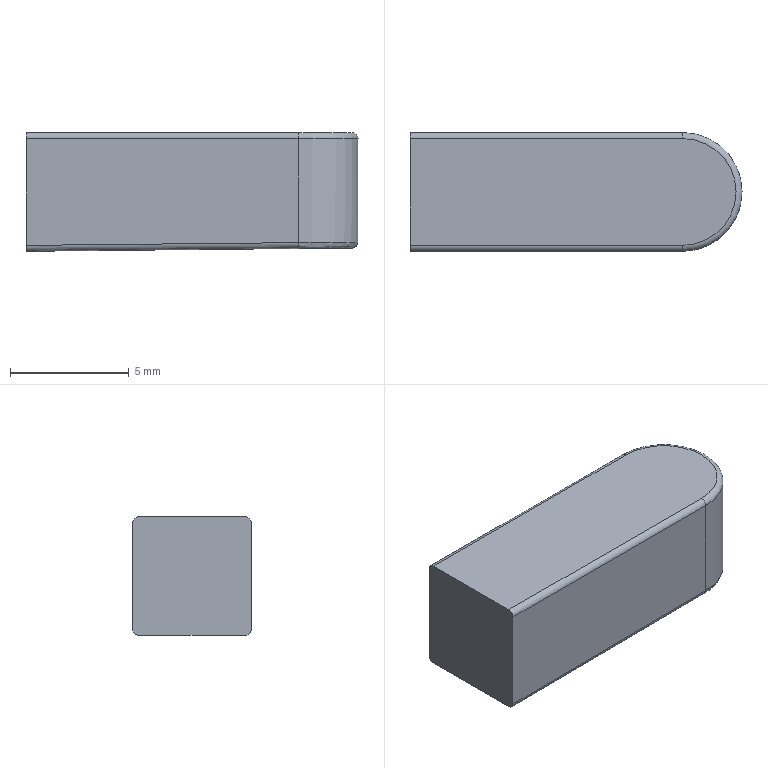Part | SolidWorks | features Cut 1, Extrusion 1, Fillet 1 | 1 solid | 12 faces | box 14 x 5 x 5 mm | volume 331.224 mm3 | plane 5 | cylinder 5 | torus 1 | spline 1 | commonest cylinder face diameters 0.5 x4 5 x1
STEP:
#1=CARTESIAN_POINT('',(-7.,-2.5,4.75));
#2=VERTEX_POINT('',#1);
#3=CARTESIAN_POINT('',(-7.,-2.5,0.25));
#4=VERTEX_POINT('',#3);
#5=CARTESIAN_POINT('',(-7.,-2.5,5.));
#6=DIRECTION('',(0.,0.,-1.));
#7=VECTOR('',#6,1000.);
#8=LINE('',#5,#7);
#9=EDGE_CURVE('',#2,#4,#8,.T.);
#10=ORIENTED_EDGE('',*,*,#9,.F.);
#11=CARTESIAN_POINT('',(-7.,-2.25,5.));
#12=VERTEX_POINT('',#11);
#13=CARTESIAN_POINT('',(-7.,-2.25,4.75));
#14=DIRECTION('',(-1.,0.,0.));
#15=DIRECTION('',(0.,0.,-1.));
#16=AXIS2_PLACEMENT_3D('',#13,#14,#15);
#17=CIRCLE('',#16,0.25);
#18=EDGE_CURVE('',#2,#12,#17,.T.);
#19=ORIENTED_EDGE('',*,*,#18,.T.);
#20=CARTESIAN_POINT('',(-7.,2.25,5.));
#21=VERTEX_POINT('',#20);
#22=CARTESIAN_POINT('',(-7.,2.5,5.));
#23=DIRECTION('',(0.,-1.,0.));
#24=VECTOR('',#23,1000.);
#25=LINE('',#22,#24);
#26=EDGE_CURVE('',#21,#12,#25,.T.);
#27=ORIENTED_EDGE('',*,*,#26,.F.);
#28=CARTESIAN_POINT('',(-7.,2.5,4.75));
#29=VERTEX_POINT('',#28);
#30=CARTESIAN_POINT('',(-7.,2.25,4.75));
#31=DIRECTION('',(-1.,0.,0.));
#32=DIRECTION('',(0.,0.,-1.));
#33=AXIS2_PLACEMENT_3D('',#30,#31,#32);
#34=CIRCLE('',#33,0.25);
#35=EDGE_CURVE('',#21,#29,#34,.T.);
#36=ORIENTED_EDGE('',*,*,#35,.T.);
#37=CARTESIAN_POINT('',(-7.,2.5,0.25));
#38=VERTEX_POINT('',#37);
#39=CARTESIAN_POINT('',(-7.,2.5,5.));
#40=DIRECTION('',(0.,0.,-1.));
#41=VECTOR('',#40,1000.);
#42=LINE('',#39,#41);
#43=EDGE_CURVE('',#29,#38,#42,.T.);
#44=ORIENTED_EDGE('',*,*,#43,.T.);
#45=CARTESIAN_POINT('',(-7.,2.25,0.));
#46=VERTEX_POINT('',#45);
#47=CARTESIAN_POINT('',(-7.,2.5,0.25));
#48=CARTESIAN_POINT('',(-7.,2.5,0.1036));
#49=CARTESIAN_POINT('',(-7.,2.396,0.));
#50=CARTESIAN_POINT('',(-7.,2.25,0.));
#51=(BOUNDED_CURVE()B_SPLINE_CURVE(3,(#47,#48,#49,#50),.UNSPECIFIED.,.F.,.T.)B_SPLINE_CURVE_WITH_KNOTS((4,4),(1.571,3.142),.UNSPECIFIED.)CURVE()GEOMETRIC_REPRESENTATION_ITEM()RATIONAL_B_SPLINE_CURVE((1.,0.8047,0.8047,1.))REPRESENTATION_ITEM(''));
#52=EDGE_CURVE('',#38,#46,#51,.T.);
#53=ORIENTED_EDGE('',*,*,#52,.T.);
#54=CARTESIAN_POINT('',(-7.,-2.25,0.));
#55=VERTEX_POINT('',#54);
#56=CARTESIAN_POINT('',(-7.,2.5,0.));
#57=DIRECTION('',(0.,-1.,0.));
#58=VECTOR('',#57,1000.);
#59=LINE('',#56,#58);
#60=EDGE_CURVE('',#46,#55,#59,.T.);
#61=ORIENTED_EDGE('',*,*,#60,.T.);
#62=CARTESIAN_POINT('',(-7.,-2.25,0.));
#63=CARTESIAN_POINT('',(-7.,-2.396,0.));
#64=CARTESIAN_POINT('',(-7.,-2.5,0.1036));
#65=CARTESIAN_POINT('',(-7.,-2.5,0.25));
#66=(BOUNDED_CURVE()B_SPLINE_CURVE(3,(#62,#63,#64,#65),.UNSPECIFIED.,.F.,.T.)B_SPLINE_CURVE_WITH_KNOTS((4,4),(3.142,4.712),.UNSPECIFIED.)CURVE()GEOMETRIC_REPRESENTATION_ITEM()RATIONAL_B_SPLINE_CURVE((1.,0.8047,0.8047,1.))REPRESENTATION_ITEM(''));
#67=EDGE_CURVE('',#55,#4,#66,.T.);
#68=ORIENTED_EDGE('',*,*,#67,.T.);
#69=EDGE_LOOP('',(#10,#19,#27,#36,#44,#53,#61,#68));
#70=FACE_OUTER_BOUND('',#69,.T.);
#71=CARTESIAN_POINT('',(-7.,2.5,5.));
#72=DIRECTION('',(1.,0.,0.));
#73=DIRECTION('',(0.,0.,-1.));
#74=AXIS2_PLACEMENT_3D('',#71,#72,#73);
#75=PLANE('',#74);
#76=ADVANCED_FACE('',(#70),#75,.F.);
#77=CARTESIAN_POINT('',(4.5,-2.5,4.75));
#78=VERTEX_POINT('',#77);
#79=CARTESIAN_POINT('',(4.5,-2.5,0.365));
#80=VERTEX_POINT('',#79);
#81=CARTESIAN_POINT('',(4.5,-2.5,5.));
#82=DIRECTION('',(0.,0.,-1.));
#83=VECTOR('',#82,1000.);
#84=LINE('',#81,#83);
#85=EDGE_CURVE('',#78,#80,#84,.T.);
#86=ORIENTED_EDGE('',*,*,#85,.F.);
#87=CARTESIAN_POINT('',(4.5,-2.5,4.75));
#88=DIRECTION('',(-1.,0.,0.));
#89=VECTOR('',#88,1000.);
#90=LINE('',#87,#89);
#91=EDGE_CURVE('',#78,#2,#90,.T.);
#92=ORIENTED_EDGE('',*,*,#91,.T.);
#93=ORIENTED_EDGE('',*,*,#9,.T.);
#94=CARTESIAN_POINT('',(4.546,-2.5,0.3655));
#95=DIRECTION('',(1.,0.,0.01));
#96=VECTOR('',#95,1000.);
#97=LINE('',#94,#96);
#98=EDGE_CURVE('',#4,#80,#97,.T.);
#99=ORIENTED_EDGE('',*,*,#98,.T.);
#100=EDGE_LOOP('',(#86,#92,#93,#99));
#101=FACE_OUTER_BOUND('',#100,.T.);
#102=CARTESIAN_POINT('',(4.5,-2.5,5.));
#103=DIRECTION('',(0.,1.,0.));
#104=DIRECTION('',(-1.,0.,0.));
#105=AXIS2_PLACEMENT_3D('',#102,#103,#104);
#106=PLANE('',#105);
#107=ADVANCED_FACE('',(#101),#106,.F.);
#108=CARTESIAN_POINT('',(4.5,2.5,4.75));
#109=VERTEX_POINT('',#108);
#110=CARTESIAN_POINT('',(4.5,2.5,0.365));
#111=VERTEX_POINT('',#110);
#112=CARTESIAN_POINT('',(4.5,2.5,5.));
#113=DIRECTION('',(0.,0.,-1.));
#114=VECTOR('',#113,1000.);
#115=LINE('',#112,#114);
#116=EDGE_CURVE('',#109,#111,#115,.T.);
#117=ORIENTED_EDGE('',*,*,#116,.F.);
#118=CARTESIAN_POINT('',(4.5,0.,4.75));
#119=DIRECTION('',(0.,0.,-1.));
#120=DIRECTION('',(-1.,0.,0.));
#121=AXIS2_PLACEMENT_3D('',#118,#119,#120);
#122=CIRCLE('',#121,2.5);
#123=EDGE_CURVE('',#109,#78,#122,.T.);
#124=ORIENTED_EDGE('',*,*,#123,.T.);
#125=ORIENTED_EDGE('',*,*,#85,.T.);
#126=CARTESIAN_POINT('',(4.5,-2.5,0.365));
#127=CARTESIAN_POINT('',(9.5,-2.5,0.41));
#128=CARTESIAN_POINT('',(9.5,2.5,0.41));
#129=CARTESIAN_POINT('',(4.5,2.5,0.365));
#130=(BOUNDED_CURVE()B_SPLINE_CURVE(3,(#126,#127,#128,#129),.UNSPECIFIED.,.F.,.F.)B_SPLINE_CURVE_WITH_KNOTS((4,4),(1.571,4.712),.UNSPECIFIED.)CURVE()GEOMETRIC_REPRESENTATION_ITEM()RATIONAL_B_SPLINE_CURVE((1.,0.3333,0.3333,1.))REPRESENTATION_ITEM(''));
#131=EDGE_CURVE('',#80,#111,#130,.T.);
#132=ORIENTED_EDGE('',*,*,#131,.T.);
#133=EDGE_LOOP('',(#117,#124,#125,#132));
#134=FACE_OUTER_BOUND('',#133,.T.);
#135=CARTESIAN_POINT('',(4.5,0.,5.));
#136=DIRECTION('',(0.,0.,-1.));
#137=DIRECTION('',(-1.,0.,0.));
#138=AXIS2_PLACEMENT_3D('',#135,#136,#137);
#139=CYLINDRICAL_SURFACE('',#138,2.5);
#140=ADVANCED_FACE('',(#134),#139,.T.);
#141=ORIENTED_EDGE('',*,*,#116,.T.);
#142=CARTESIAN_POINT('',(-6.953,2.5,0.2505));
#143=DIRECTION('',(-1.,0.,-0.01));
#144=VECTOR('',#143,1000.);
#145=LINE('',#142,#144);
#146=EDGE_CURVE('',#111,#38,#145,.T.);
#147=ORIENTED_EDGE('',*,*,#146,.T.);
#148=ORIENTED_EDGE('',*,*,#43,.F.);
#149=CARTESIAN_POINT('',(-7.,2.5,4.75));
#150=DIRECTION('',(1.,0.,0.));
#151=VECTOR('',#150,1000.);
#152=LINE('',#149,#151);
#153=EDGE_CURVE('',#29,#109,#152,.T.);
#154=ORIENTED_EDGE('',*,*,#153,.T.);
#155=EDGE_LOOP('',(#141,#147,#148,#154));
#156=FACE_OUTER_BOUND('',#155,.T.);
#157=CARTESIAN_POINT('',(-7.,2.5,5.));
#158=DIRECTION('',(0.,-1.,0.));
#159=DIRECTION('',(1.,0.,0.));
#160=AXIS2_PLACEMENT_3D('',#157,#158,#159);
#161=PLANE('',#160);
#162=ADVANCED_FACE('',(#156),#161,.F.);
#163=ORIENTED_EDGE('',*,*,#26,.T.);
#164=CARTESIAN_POINT('',(4.5,-2.25,5.));
#165=VERTEX_POINT('',#164);
#166=CARTESIAN_POINT('',(4.5,-2.25,5.));
#167=DIRECTION('',(1.,0.,0.));
#168=VECTOR('',#167,1000.);
#169=LINE('',#166,#168);
#170=EDGE_CURVE('',#12,#165,#169,.T.);
#171=ORIENTED_EDGE('',*,*,#170,.T.);
#172=CARTESIAN_POINT('',(4.5,2.25,5.));
#173=VERTEX_POINT('',#172);
#174=CARTESIAN_POINT('',(4.5,0.,5.));
#175=DIRECTION('',(0.,0.,1.));
#176=DIRECTION('',(-1.,0.,0.));
#177=AXIS2_PLACEMENT_3D('',#174,#175,#176);
#178=CIRCLE('',#177,2.25);
#179=EDGE_CURVE('',#165,#173,#178,.T.);
#180=ORIENTED_EDGE('',*,*,#179,.T.);
#181=CARTESIAN_POINT('',(4.5,2.25,5.));
#182=DIRECTION('',(-1.,0.,0.));
#183=VECTOR('',#182,1000.);
#184=LINE('',#181,#183);
#185=EDGE_CURVE('',#173,#21,#184,.T.);
#186=ORIENTED_EDGE('',*,*,#185,.T.);
#187=EDGE_LOOP('',(#163,#171,#180,#186));
#188=FACE_OUTER_BOUND('',#187,.T.);
#189=CARTESIAN_POINT('',(4.5,0.,5.));
#190=DIRECTION('',(0.,0.,-1.));
#191=DIRECTION('',(-1.,0.,0.));
#192=AXIS2_PLACEMENT_3D('',#189,#190,#191);
#193=PLANE('',#192);
#194=ADVANCED_FACE('',(#188),#193,.F.);
#195=ORIENTED_EDGE('',*,*,#60,.F.);
#196=CARTESIAN_POINT('',(4.502,2.25,0.115));
#197=VERTEX_POINT('',#196);
#198=CARTESIAN_POINT('',(-7.,2.25,0.));
#199=DIRECTION('',(1.,0.,0.01));
#200=VECTOR('',#199,1000.);
#201=LINE('',#198,#200);
#202=EDGE_CURVE('',#46,#197,#201,.T.);
#203=ORIENTED_EDGE('',*,*,#202,.T.);
#204=CARTESIAN_POINT('',(4.502,-2.25,0.115));
#205=VERTEX_POINT('',#204);
#206=CARTESIAN_POINT('',(4.502,2.25,0.115));
#207=CARTESIAN_POINT('',(9.002,2.25,0.16));
#208=CARTESIAN_POINT('',(9.002,-2.25,0.16));
#209=CARTESIAN_POINT('',(4.502,-2.25,0.115));
#210=(BOUNDED_CURVE()B_SPLINE_CURVE(3,(#206,#207,#208,#209),.UNSPECIFIED.,.F.,.T.)B_SPLINE_CURVE_WITH_KNOTS((4,4),(1.571,4.712),.UNSPECIFIED.)CURVE()GEOMETRIC_REPRESENTATION_ITEM()RATIONAL_B_SPLINE_CURVE((1.,0.3333,0.3333,1.))REPRESENTATION_ITEM(''));
#211=EDGE_CURVE('',#197,#205,#210,.T.);
#212=ORIENTED_EDGE('',*,*,#211,.T.);
#213=CARTESIAN_POINT('',(-7.,-2.25,0.));
#214=DIRECTION('',(-1.,0.,-0.01));
#215=VECTOR('',#214,1000.);
#216=LINE('',#213,#215);
#217=EDGE_CURVE('',#205,#55,#216,.T.);
#218=ORIENTED_EDGE('',*,*,#217,.T.);
#219=EDGE_LOOP('',(#195,#203,#212,#218));
#220=FACE_OUTER_BOUND('',#219,.T.);
#221=CARTESIAN_POINT('',(-7.,-2.5,0.));
#222=DIRECTION('',(-0.01,0.,1.));
#223=DIRECTION('',(1.,0.,0.01));
#224=AXIS2_PLACEMENT_3D('',#221,#222,#223);
#225=PLANE('',#224);
#226=ADVANCED_FACE('',(#220),#225,.F.);
#227=ORIENTED_EDGE('',*,*,#35,.F.);
#228=ORIENTED_EDGE('',*,*,#185,.F.);
#229=CARTESIAN_POINT('',(4.5,2.25,4.75));
#230=DIRECTION('',(1.,0.,0.));
#231=DIRECTION('',(0.,0.,-1.));
#232=AXIS2_PLACEMENT_3D('',#229,#230,#231);
#233=CIRCLE('',#232,0.25);
#234=EDGE_CURVE('',#109,#173,#233,.T.);
#235=ORIENTED_EDGE('',*,*,#234,.F.);
#236=ORIENTED_EDGE('',*,*,#153,.F.);
#237=EDGE_LOOP('',(#227,#228,#235,#236));
#238=FACE_OUTER_BOUND('',#237,.T.);
#239=CARTESIAN_POINT('',(4.5,2.25,4.75));
#240=DIRECTION('',(-1.,0.,0.));
#241=DIRECTION('',(0.,-1.,0.));
#242=AXIS2_PLACEMENT_3D('',#239,#240,#241);
#243=CYLINDRICAL_SURFACE('',#242,0.25);
#244=ADVANCED_FACE('',(#238),#243,.T.);
#245=ORIENTED_EDGE('',*,*,#234,.T.);
#246=ORIENTED_EDGE('',*,*,#179,.F.);
#247=CARTESIAN_POINT('',(4.5,-2.25,4.75));
#248=DIRECTION('',(-1.,0.,0.));
#249=DIRECTION('',(0.,0.,1.));
#250=AXIS2_PLACEMENT_3D('',#247,#248,#249);
#251=CIRCLE('',#250,0.25);
#252=EDGE_CURVE('',#78,#165,#251,.T.);
#253=ORIENTED_EDGE('',*,*,#252,.F.);
#254=ORIENTED_EDGE('',*,*,#123,.F.);
#255=EDGE_LOOP('',(#245,#246,#253,#254));
#256=FACE_OUTER_BOUND('',#255,.T.);
#257=CARTESIAN_POINT('',(4.5,0.,4.75));
#258=DIRECTION('',(0.,0.,-1.));
#259=DIRECTION('',(-1.,0.,0.));
#260=AXIS2_PLACEMENT_3D('',#257,#258,#259);
#261=TOROIDAL_SURFACE('',#260,2.25,0.25);
#262=ADVANCED_FACE('',(#256),#261,.T.);
#263=ORIENTED_EDGE('',*,*,#18,.F.);
#264=ORIENTED_EDGE('',*,*,#91,.F.);
#265=ORIENTED_EDGE('',*,*,#252,.T.);
#266=ORIENTED_EDGE('',*,*,#170,.F.);
#267=EDGE_LOOP('',(#263,#264,#265,#266));
#268=FACE_OUTER_BOUND('',#267,.T.);
#269=CARTESIAN_POINT('',(4.5,-2.25,4.75));
#270=DIRECTION('',(1.,0.,0.));
#271=DIRECTION('',(0.,1.,0.));
#272=AXIS2_PLACEMENT_3D('',#269,#270,#271);
#273=CYLINDRICAL_SURFACE('',#272,0.25);
#274=ADVANCED_FACE('',(#268),#273,.T.);
#275=ORIENTED_EDGE('',*,*,#67,.F.);
#276=ORIENTED_EDGE('',*,*,#217,.F.);
#277=CARTESIAN_POINT('',(4.5,-2.25,0.365));
#278=DIRECTION('',(1.,0.,0.01));
#279=DIRECTION('',(0.01,0.,-1.));
#280=AXIS2_PLACEMENT_3D('',#277,#278,#279);
#281=CIRCLE('',#280,0.25);
#282=EDGE_CURVE('',#80,#205,#281,.T.);
#283=ORIENTED_EDGE('',*,*,#282,.F.);
#284=ORIENTED_EDGE('',*,*,#98,.F.);
#285=EDGE_LOOP('',(#275,#276,#283,#284));
#286=FACE_OUTER_BOUND('',#285,.T.);
#287=CARTESIAN_POINT('',(4.546,-2.25,0.3655));
#288=DIRECTION('',(1.,0.,0.01));
#289=DIRECTION('',(0.01,0.,-1.));
#290=AXIS2_PLACEMENT_3D('',#287,#288,#289);
#291=CYLINDRICAL_SURFACE('',#290,0.25);
#292=ADVANCED_FACE('',(#286),#291,.T.);
#293=ORIENTED_EDGE('',*,*,#282,.T.);
#294=ORIENTED_EDGE('',*,*,#211,.F.);
#295=CARTESIAN_POINT('',(4.5,2.25,0.365));
#296=DIRECTION('',(-1.,0.,-0.01));
#297=DIRECTION('',(-0.01,0.,1.));
#298=AXIS2_PLACEMENT_3D('',#295,#296,#297);
#299=CIRCLE('',#298,0.25);
#300=EDGE_CURVE('',#111,#197,#299,.T.);
#301=ORIENTED_EDGE('',*,*,#300,.F.);
#302=ORIENTED_EDGE('',*,*,#131,.F.);
#303=EDGE_LOOP('',(#293,#294,#301,#302));
#304=FACE_OUTER_BOUND('',#303,.T.);
#305=CARTESIAN_POINT('',(4.502,-2.25,0.115));
#306=CARTESIAN_POINT('',(4.502,-2.5,0.115));
#307=CARTESIAN_POINT('',(4.5,-2.5,0.365));
#308=CARTESIAN_POINT('',(4.797,-2.25,0.118));
#309=CARTESIAN_POINT('',(4.83,-2.5,0.1183));
#310=CARTESIAN_POINT('',(4.827,-2.5,0.368));
#311=CARTESIAN_POINT('',(5.091,-2.191,0.1209));
#312=CARTESIAN_POINT('',(5.157,-2.434,0.1216));
#313=CARTESIAN_POINT('',(5.154,-2.435,0.3709));
#314=CARTESIAN_POINT('',(5.636,-1.966,0.1264));
#315=CARTESIAN_POINT('',(5.761,-2.183,0.1276));
#316=CARTESIAN_POINT('',(5.759,-2.184,0.3763));
#317=CARTESIAN_POINT('',(5.885,-1.799,0.1289));
#318=CARTESIAN_POINT('',(6.038,-1.998,0.1304));
#319=CARTESIAN_POINT('',(6.036,-1.999,0.3788));
#320=CARTESIAN_POINT('',(6.302,-1.383,0.133));
#321=CARTESIAN_POINT('',(6.5,-1.535,0.135));
#322=CARTESIAN_POINT('',(6.499,-1.536,0.383));
#323=CARTESIAN_POINT('',(6.469,-1.133,0.1347));
#324=CARTESIAN_POINT('',(6.685,-1.258,0.1369));
#325=CARTESIAN_POINT('',(6.684,-1.259,0.3847));
#326=CARTESIAN_POINT('',(6.694,-0.5889,0.1369));
#327=CARTESIAN_POINT('',(6.935,-0.6538,0.1394));
#328=CARTESIAN_POINT('',(6.935,-0.6544,0.3869));
#329=CARTESIAN_POINT('',(6.752,-0.2945,0.1375));
#330=CARTESIAN_POINT('',(7.,-0.3269,0.14));
#331=CARTESIAN_POINT('',(7.,-0.3272,0.3875));
#332=CARTESIAN_POINT('',(6.752,0.2945,0.1375));
#333=CARTESIAN_POINT('',(7.,0.3269,0.14));
#334=CARTESIAN_POINT('',(7.,0.3272,0.3875));
#335=CARTESIAN_POINT('',(6.694,0.5889,0.1369));
#336=CARTESIAN_POINT('',(6.935,0.6538,0.1394));
#337=CARTESIAN_POINT('',(6.935,0.6544,0.3869));
#338=CARTESIAN_POINT('',(6.469,1.133,0.1347));
#339=CARTESIAN_POINT('',(6.685,1.258,0.1369));
#340=CARTESIAN_POINT('',(6.684,1.259,0.3847));
#341=CARTESIAN_POINT('',(6.302,1.383,0.133));
#342=CARTESIAN_POINT('',(6.5,1.535,0.135));
#343=CARTESIAN_POINT('',(6.499,1.536,0.383));
#344=CARTESIAN_POINT('',(5.885,1.799,0.1289));
#345=CARTESIAN_POINT('',(6.038,1.998,0.1304));
#346=CARTESIAN_POINT('',(6.036,1.999,0.3788));
#347=CARTESIAN_POINT('',(5.636,1.966,0.1264));
#348=CARTESIAN_POINT('',(5.761,2.183,0.1276));
#349=CARTESIAN_POINT('',(5.759,2.184,0.3763));
#350=CARTESIAN_POINT('',(5.091,2.191,0.1209));
#351=CARTESIAN_POINT('',(5.157,2.434,0.1216));
#352=CARTESIAN_POINT('',(5.154,2.435,0.3709));
#353=CARTESIAN_POINT('',(4.797,2.25,0.118));
#354=CARTESIAN_POINT('',(4.83,2.5,0.1183));
#355=CARTESIAN_POINT('',(4.827,2.5,0.368));
#356=CARTESIAN_POINT('',(4.502,2.25,0.115));
#357=CARTESIAN_POINT('',(4.502,2.5,0.115));
#358=CARTESIAN_POINT('',(4.5,2.5,0.365));
#359=(BOUNDED_SURFACE()B_SPLINE_SURFACE(3,2,((#305,#306,#307),(#308,#309,#310),(#311,#312,#313),(#314,#315,#316),(#317,#318,#319),(#320,#321,#322),(#323,#324,#325),(#326,#327,#328),(#329,#330,#331),(#332,#333,#334),(#335,#336,#337),(#338,#339,#340),(#341,#342,#343),(#344,#345,#346),(#347,#348,#349),(#350,#351,#352),(#353,#354,#355),(#356,#357,#358)),.UNSPECIFIED.,.F.,.F.,.F.)B_SPLINE_SURFACE_WITH_KNOTS((4,2,2,2,2,2,2,2,4),(3,3),(1.571,1.963,2.356,2.749,3.142,3.534,3.927,4.32,4.712),(0.,1.),.UNSPECIFIED.)GEOMETRIC_REPRESENTATION_ITEM()RATIONAL_B_SPLINE_SURFACE(((1.,0.7071,1.),(1.,0.7076,1.),(1.,0.708,1.),(1.,0.7089,1.),(1.,0.7093,1.),(1.,0.7099,1.),(1.,0.7102,1.),(1.,0.7105,1.),(1.,0.7106,1.),(1.,0.7106,1.),(1.,0.7105,1.),(1.,0.7102,1.),(1.,0.7099,1.),(1.,0.7093,1.),(1.,0.7089,1.),(1.,0.708,1.),(1.,0.7076,1.),(1.,0.7071,1.)))REPRESENTATION_ITEM('')SURFACE());
#360=ADVANCED_FACE('',(#304),#359,.T.);
#361=ORIENTED_EDGE('',*,*,#52,.F.);
#362=ORIENTED_EDGE('',*,*,#146,.F.);
#363=ORIENTED_EDGE('',*,*,#300,.T.);
#364=ORIENTED_EDGE('',*,*,#202,.F.);
#365=EDGE_LOOP('',(#361,#362,#363,#364));
#366=FACE_OUTER_BOUND('',#365,.T.);
#367=CARTESIAN_POINT('',(-7.002,2.25,0.25));
#368=DIRECTION('',(1.,0.,0.01));
#369=DIRECTION('',(0.01,0.,-1.));
#370=AXIS2_PLACEMENT_3D('',#367,#368,#369);
#371=CYLINDRICAL_SURFACE('',#370,0.25);
#372=ADVANCED_FACE('',(#366),#371,.T.);
#373=CLOSED_SHELL('',(#76,#107,#140,#162,#194,#226,#244,#262,#274,#292,#360,#372));
#374=MANIFOLD_SOLID_BREP('',#373);
#375=CARTESIAN_POINT('',(0.,0.,0.));
#376=DIRECTION('',(0.,0.,1.));
#377=DIRECTION('',(1.,0.,0.));
#378=AXIS2_PLACEMENT_3D('',#375,#376,#377);
#379=(LENGTH_UNIT()NAMED_UNIT(*)SI_UNIT(.MILLI.,.METRE.));
#380=UNCERTAINTY_MEASURE_WITH_UNIT(LENGTH_MEASURE(0.00001),#379,'','');
#381=(NAMED_UNIT(*)PLANE_ANGLE_UNIT()SI_UNIT($,.RADIAN.));
#382=(NAMED_UNIT(*)SI_UNIT($,.STERADIAN.)SOLID_ANGLE_UNIT());
#383=(GEOMETRIC_REPRESENTATION_CONTEXT(3)GLOBAL_UNCERTAINTY_ASSIGNED_CONTEXT((#380))GLOBAL_UNIT_ASSIGNED_CONTEXT((#379,#381,#382))REPRESENTATION_CONTEXT('',''));
#384=ADVANCED_BREP_SHAPE_REPRESENTATION('',(#374,#378),#383);